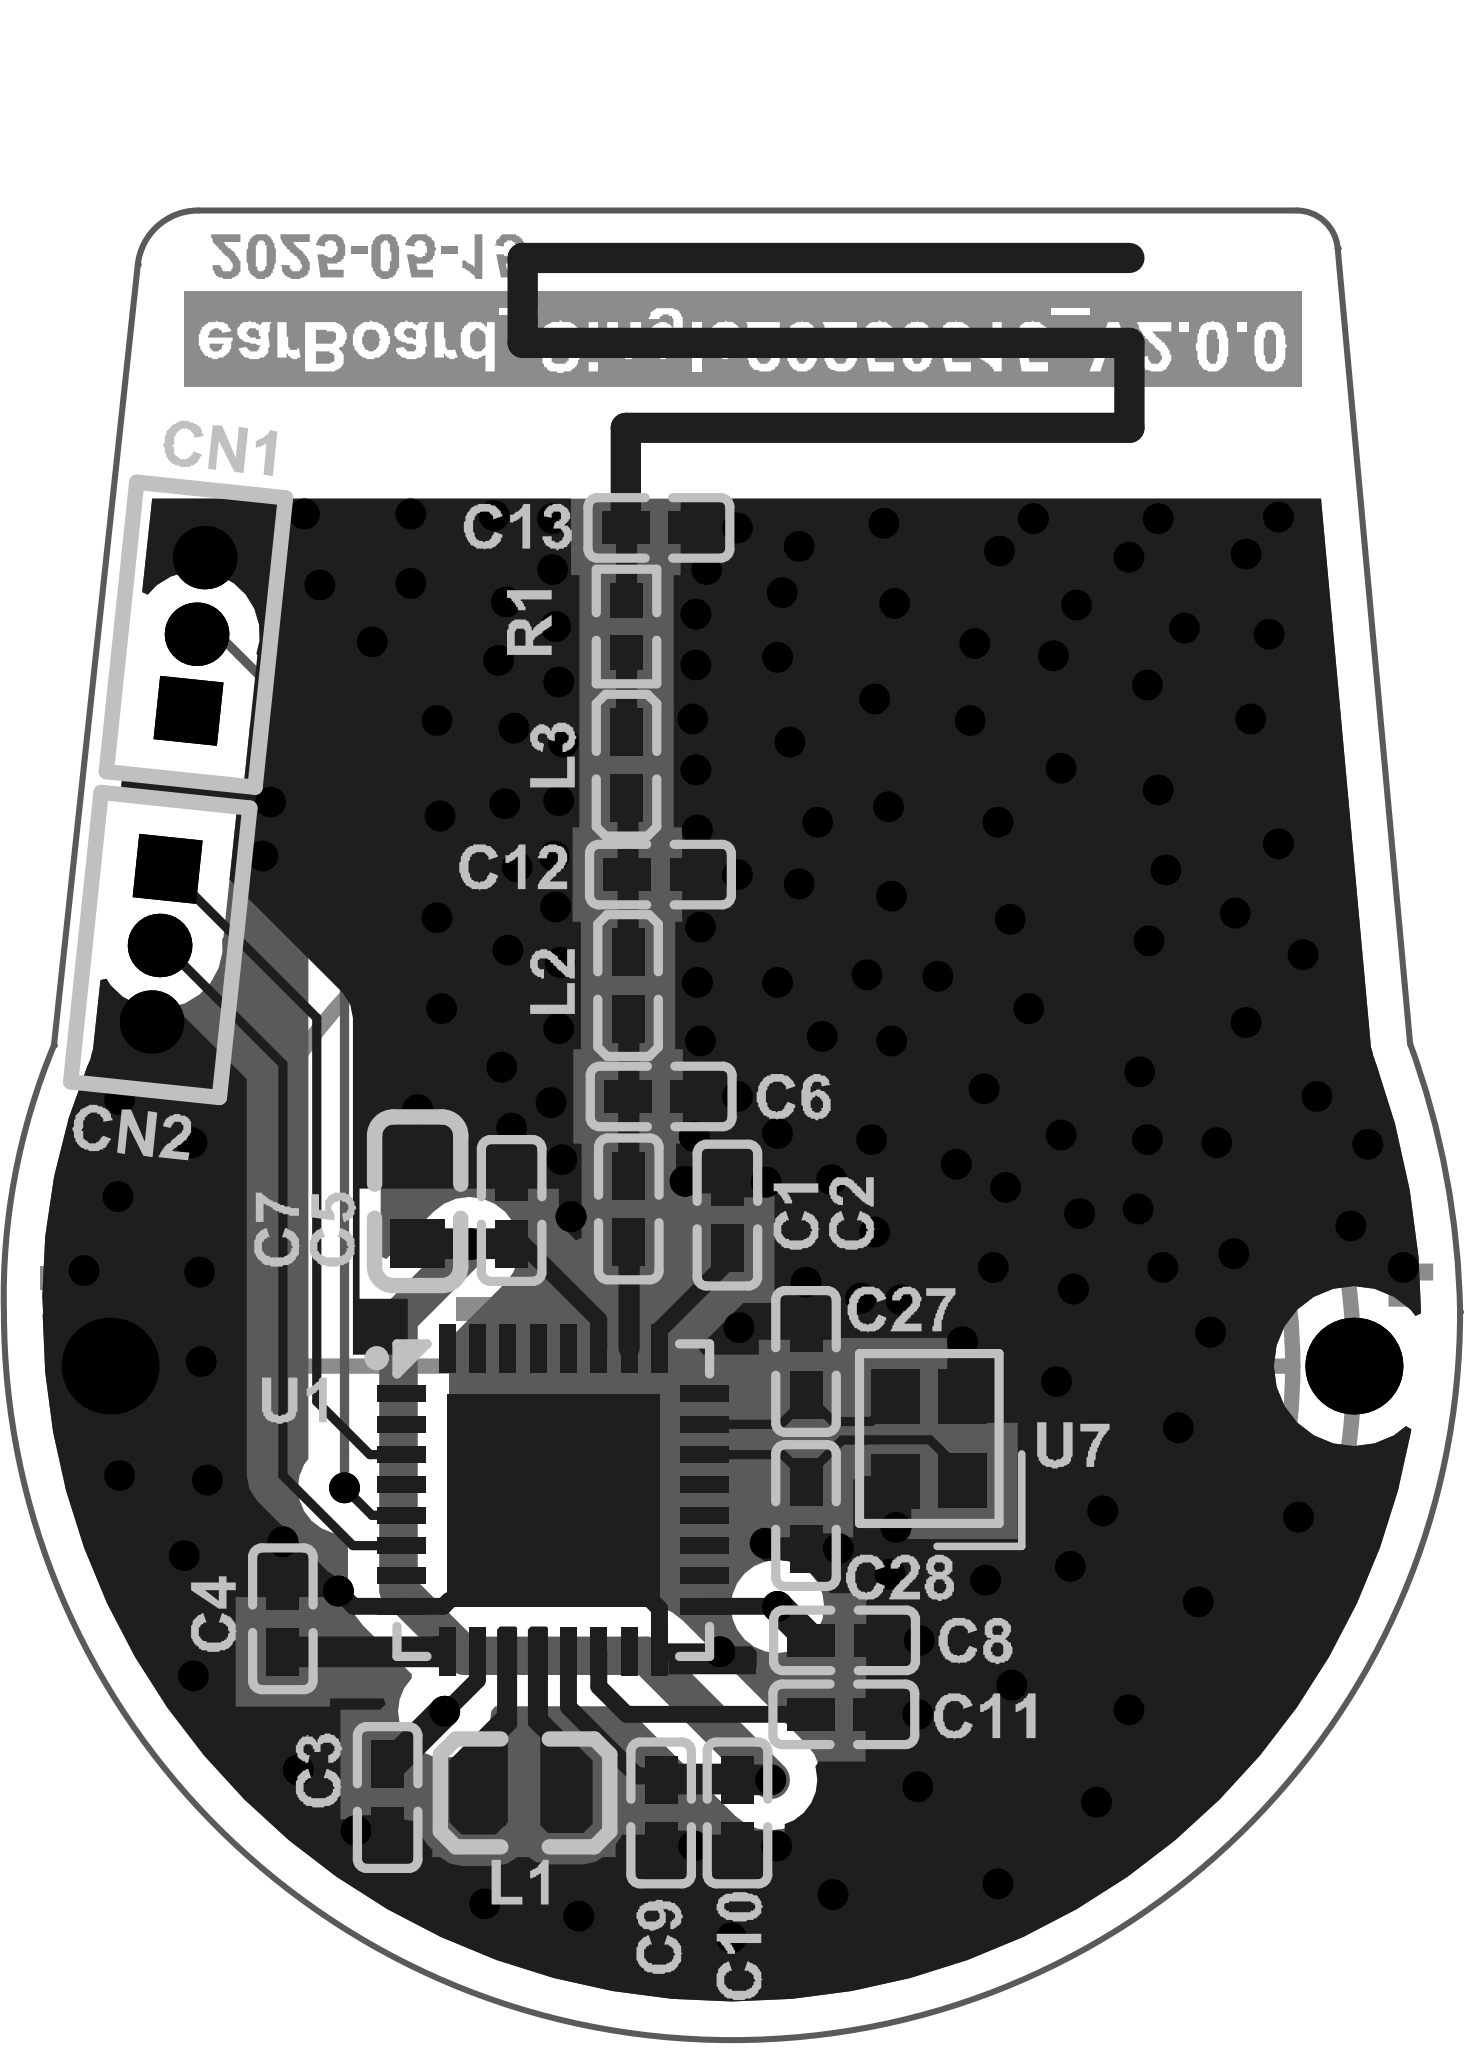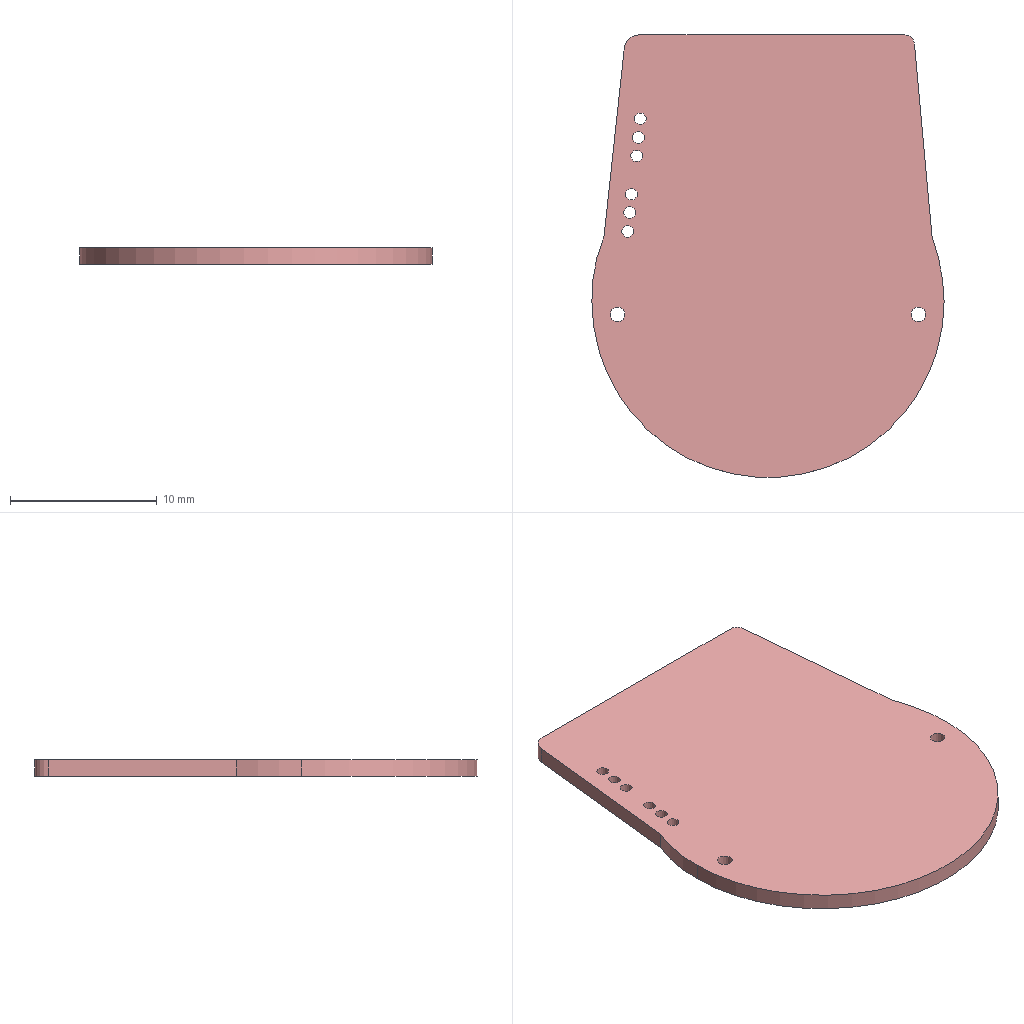Circuit board layout | Altium Designer | box 24 x 30.1 x 1.1 mm
Layer stack:
# Altium Designer layer stack of  (unit mm; dielectric type: 0 none, 1 core, 2 prepreg, 3 surface material)
index,name,kind,layer,copper_thickness_mm,dielectric_type,dielectric_thickness_mm,dielectric_material,dielectric_constant
0,Top Paste,other,,,,,,
1,Top Overlay,other,,,,,,
2,Top Solder,dielectric,,,3,0.0102,Solder Resist,3.5
3,Top Layer,copper,Top Layer,0.0356,,,,
4,Dielectric1,dielectric,,,1,0.32,FR-4,4.8
5,GND,copper,GND,0.0356,,,,
6,Dielectric2,dielectric,,,2,0.32,FR-4,4.8
7,POWER,copper,POWER,0.0356,,,,
8,Dielectric3,dielectric,,,1,0.32,FR-4,4.8
9,Bottom Layer,copper,Bottom Layer,0.0356,,,,
10,Bottom Solder,dielectric,,,3,0.0102,Solder Resist,3.5
11,Bottom Overlay,other,,,,,,
12,Bottom Paste,other,,,,,,
# drill layer pairs: low layer,high layer
drill_pair,Top Layer,Bottom Layer
Part placement:
Designator,Comment,Layer,Footprint,Center-X(mm),Center-Y(mm),Rotation
R1,,TopLayer,R0402,10.262,11.303,90
L3,2.4nH,TopLayer,L0402,10.262,9.017,90
L2,2.4nH,TopLayer,L0402,10.287,5.385,90
C13,2pF,TopLayer,C0402,10.795,12.929,180
C12,2pF,TopLayer,C0402,10.82,7.214,180
C6,2pF,TopLayer,C0402,10.832,3.556,180
C1,220pF,TopLayer,C0402,10.299,1.702,90
U7,24MHz,TopLayer,JWT1238,15.252,-2.083,90
U1,TLSR8355F512ET32,TopLayer,TQFN-32_L5.0-W5.0-P0.50-BL-EP3.5,9.054,-3.099,270
C28,12pF,TopLayer,C0402,13.22,-3.353,270
C27,12pF,TopLayer,C0402,13.22,-0.8128,90
U2,Q&J CR2032 20-6*9,TopLayer,BAT-TH_CR2032,12,-0.889,180
CN2,,TopLayer,HDR-TH_3P-P1.27-V-M-A,2.565,6.045,264
CN1,,TopLayer,HDR-TH_3P-P1.27-V-M-A,3.175,11.176,84
L1,4.7uH,TopLayer,IND-SMD_L1.8-W1.2,8.572,-7.925,360
C10,0.1uF,TopLayer,C0402,12.09,-8.255,90
C9,2.2uF,TopLayer,C0402,10.832,-8.255,90
C8,1uF,TopLayer,C0402,13.855,-5.41,360
C7,0.1uF,TopLayer,C0603,6.819,1.829,270
C11,1uF,TopLayer,C0402,13.843,-6.629,180
C5,1uF,TopLayer,C0402,8.368,1.676,270
C4,1uF,TopLayer,C0402,4.597,-5.055,270
C3,1uF,TopLayer,C0402,6.325,-8.001,90
C2,1uF,TopLayer,C0402,11.924,1.6,270
Pad and via stacks:
# Altium Designer via and pad stacks of  (unit mm). Each distinct definition once, with the count of objects using it.
# via: kind,start_layer,end_layer,hole_mm,diameter_mm,mode(0 simple;1 top-mid-bottom;2 full stack),diameter_per_layer,count,example_net
# pad: kind,layer,hole_mm,hole_type(0 round;1 square;2 slot),plating,top_size,top_shape(1 round;2 rect;3 octagon;9 rounded rect),mid_size,bottom_size,mode,footprint,size_per_layer,count,example
pad,Top Layer,0,0,plated,0.5657x0.54,2,0.5657x0.54,0.5657x0.54,0,R0402,,2,R1.2
pad,Top Layer,0,0,plated,0.7901x0.54,2,0.7901x0.54,0.7901x0.54,0,C0402,,28,C1.2
pad,Top Layer,0,0,plated,0.7901x0.54,2,0.7901x0.54,0.7901x0.54,0,L0402,,4,L3.2
pad,Top Layer,0,0,plated,0.9x0.8,2,0.9x0.8,0.9x0.8,0,JWT1238,,4,U7.4
pad,Top Layer,0,0,plated,3.5x3.5,2,3.5x3.5,3.5x3.5,0,TQFN-32_L5.0-W5.0-P0.50-BL-EP3.5,,1,U1.33
pad,Top Layer,0,0,plated,0.8x0.28,2,0.8x0.28,0.8x0.28,0,TQFN-32_L5.0-W5.0-P0.50-BL-EP3.5,,16,U1.32
pad,Top Layer,0,0,plated,0.28x0.8,2,0.28x0.8,0.28x0.8,0,TQFN-32_L5.0-W5.0-P0.50-BL-EP3.5,,16,U1.24
pad,Top Layer,0,0,plated,0.7x1.1,2,0.7x1.1,0.7x1.1,0,IND-SMD_L1.8-W1.2,,2,L1.1
pad,Top Layer,0,0,plated,0.8x0.9,2,0.8x0.9,0.8x0.9,0,C0603,,2,C7.2
pad,Multi-Layer,1,0,plated,1.6x1.6,1,1.6x1.6,1.6x1.6,0,BAT-TH_CR2032,,2,U2.1
pad,Multi-Layer,0.8,0,plated,1.05x1.05,2,1.05x1.05,1.05x1.05,0,HDR-TH_3P-P1.27-V-M-A,,2,CN2.1
pad,Multi-Layer,0.8,0,plated,1.05x1.05,1,1.05x1.05,1.05x1.05,0,HDR-TH_3P-P1.27-V-M-A,,4,CN2.2
via,Top Layer,Bottom Layer,0.3048,0.508,0,,177,GND
Copper pours:
name,layer,net,type(0 solid;1 hatched;2 none)
Bottom Layer-No Net,Top Layer,GND,0
Bottom Layer-No Net,Top Layer,NetL1_2,0
Bottom Layer-No Net,Top Layer,NetL1_1,0
Bottom Layer-No Net,Bottom Layer,GND,0
Design rules, without the lines most boards share:
# Altium Designer design rules of  (exported by Altium Designer, unit mm)
# columns: name | kind | enabled | priority | scope1 | scope2 | descriptor | typed fields (field=value)
Clearance_1 | 0 | enabled | 1 | inpolygon | All | Clearance Constraint (Gap=6mil) (inpolygon),(All) | gap=0.1524
SilkToSilkClearance | 55 | enabled | 1 | All | All | Silk to Silk (Clearance=0mil) (All),(All) |
SilkscreenOverComponentPads | 54 | enabled | 1 | IsPad | All | Silk To Solder Mask (Clearance=0mil) (IsPad),(All) |
MinimumSolderMaskSliver | 53 | enabled | 1 | All | All | Minimum Solder Mask Sliver (Gap=0mil) (All),(All) |
HoleToHoleClearance | 52 | enabled | 1 | All | All | Hole To Hole Clearance (Gap=0mil) (All),(All) | gap=0
DiffPairsRouting | 51 | enabled | 1 | All | All | Differential Pairs Uncoupled Length using the Gap Constraints (Min=10mil) (Max=10mil) (Prefered=10mil)  and Width Constraints (Min=15mil) (Max=15mil) (Prefered=15mil) (All) |
SolderMaskExpansion | 13 | enabled | 1 | All | All | Solder Mask Expansion (Expansion =4mil) (All) | expansion=0.1016
RoutingVias | 11 | enabled | 1 | All | All | Routing Via (MinHoleWidth=12mil) (MaxHoleWidth=12mil) (PreferredHoleWidth=12mil) (MinWidth=20mil) (MaxWidth=20mil) (PreferedWidth=20mil) (All) | via_min_hole=0.3048 via_max_hole=0.3048 via_preferred_diameter=0.508 via_preferred_hole=0.3048
Width | 2 | enabled | 1 | All | All | Width Constraint (Min=6mil) (Max=40mil) (Preferred=6mil) (All) |
PolygonConnect | 20 | enabled | 1 | All | All | Polygon Connect Rule(Direct Connect )(Conductor Width=10mil) (Relief Angle=90 Angle) (Entries=4) (Air Gap Width=10mil) (All),(All) | connect_style(0=relief,1=direct,2=none)=1 relief_conductor_width=0.254 relief_entries=4
PlaneClearance | 12 | enabled | 1 | All | All | Power Plane Clearance (Clearance =6mil) (All) | clearance=0.1524
PlaneConnect | 6 | enabled | 1 | All | All | Power Plane Connect Rule(Direct Connect )(Expansion=20mil) (Conductor Width=10mil) (Air Gap=10mil) (Entries=4) (All) | relief_conductor_width=0.254 relief_entries=4 relief_expansion=0.508
Clearance | 0 | enabled | 2 | All | All | Clearance Constraint (Gap=6mil) (All),(All) | gap=0.1524